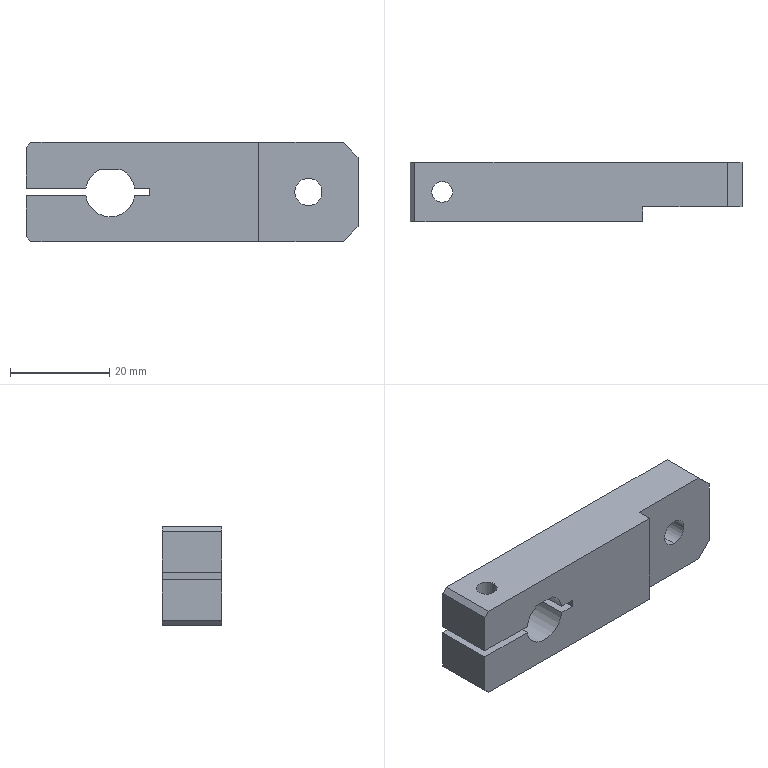Part | NX | features BREP 1 | 1 solid | 31 faces | box 67 x 12 x 20 mm | volume 12717 mm3 | plane 20 | cylinder 11 | commonest cylinder face diameters 10 x5 5.5 x4 4.2 x2
STEP:
#1=CARTESIAN_POINT('',(-22.,0.,-4.3));
#2=VERTEX_POINT('',#1);
#3=CARTESIAN_POINT('',(-32.,0.,-4.3));
#4=VERTEX_POINT('',#3);
#5=CARTESIAN_POINT('',(-27.,0.,-4.3));
#6=DIRECTION('',(0.,0.,-1.));
#7=DIRECTION('',(-1.,0.,0.));
#8=AXIS2_PLACEMENT_3D('',#5,#6,#7);
#9=CIRCLE('',#8,5.);
#10=EDGE_CURVE('',#2,#4,#9,.T.);
#11=ORIENTED_EDGE('',*,*,#10,.F.);
#12=CARTESIAN_POINT('',(-22.,0.,-10.));
#13=VERTEX_POINT('',#12);
#14=CARTESIAN_POINT('',(-22.,0.,-10.));
#15=DIRECTION('',(0.,0.,-1.));
#16=VECTOR('',#15,1000.);
#17=LINE('',#14,#16);
#18=EDGE_CURVE('',#13,#2,#17,.F.);
#19=ORIENTED_EDGE('',*,*,#18,.F.);
#20=CARTESIAN_POINT('',(-32.,0.,-10.));
#21=VERTEX_POINT('',#20);
#22=CARTESIAN_POINT('',(-27.,0.,-10.));
#23=DIRECTION('',(0.,0.,-1.));
#24=DIRECTION('',(-1.,0.,0.));
#25=AXIS2_PLACEMENT_3D('',#22,#23,#24);
#26=CIRCLE('',#25,5.);
#27=EDGE_CURVE('',#13,#21,#26,.T.);
#28=ORIENTED_EDGE('',*,*,#27,.T.);
#29=CARTESIAN_POINT('',(-32.,0.,-10.));
#30=DIRECTION('',(0.,0.,-1.));
#31=VECTOR('',#30,1000.);
#32=LINE('',#29,#31);
#33=EDGE_CURVE('',#21,#4,#32,.F.);
#34=ORIENTED_EDGE('',*,*,#33,.T.);
#35=EDGE_LOOP('',(#11,#19,#28,#34));
#36=FACE_BOUND('',#35,.T.);
#37=CARTESIAN_POINT('',(-27.,0.,-10.));
#38=DIRECTION('',(0.,0.,-1.));
#39=DIRECTION('',(1.,0.,0.));
#40=AXIS2_PLACEMENT_3D('',#37,#38,#39);
#41=CYLINDRICAL_SURFACE('',#40,5.);
#42=ADVANCED_FACE('',(#36),#41,.F.);
#43=CARTESIAN_POINT('',(-24.25,0.,-0.75));
#44=VERTEX_POINT('',#43);
#45=CARTESIAN_POINT('',(-29.75,0.,-0.75));
#46=VERTEX_POINT('',#45);
#47=CARTESIAN_POINT('',(-27.,0.,-0.75));
#48=DIRECTION('',(0.,0.,-1.));
#49=DIRECTION('',(-1.,0.,0.));
#50=AXIS2_PLACEMENT_3D('',#47,#48,#49);
#51=CIRCLE('',#50,2.75);
#52=EDGE_CURVE('',#44,#46,#51,.T.);
#53=ORIENTED_EDGE('',*,*,#52,.F.);
#54=CARTESIAN_POINT('',(-24.25,0.,-4.3));
#55=VERTEX_POINT('',#54);
#56=CARTESIAN_POINT('',(-24.25,0.,-10.));
#57=DIRECTION('',(0.,0.,-1.));
#58=VECTOR('',#57,1000.);
#59=LINE('',#56,#58);
#60=EDGE_CURVE('',#55,#44,#59,.F.);
#61=ORIENTED_EDGE('',*,*,#60,.F.);
#62=CARTESIAN_POINT('',(-29.75,0.,-4.3));
#63=VERTEX_POINT('',#62);
#64=CARTESIAN_POINT('',(-27.,0.,-4.3));
#65=DIRECTION('',(0.,0.,-1.));
#66=DIRECTION('',(-1.,0.,0.));
#67=AXIS2_PLACEMENT_3D('',#64,#65,#66);
#68=CIRCLE('',#67,2.75);
#69=EDGE_CURVE('',#55,#63,#68,.T.);
#70=ORIENTED_EDGE('',*,*,#69,.T.);
#71=CARTESIAN_POINT('',(-29.75,0.,-10.));
#72=DIRECTION('',(0.,0.,-1.));
#73=VECTOR('',#72,1000.);
#74=LINE('',#71,#73);
#75=EDGE_CURVE('',#63,#46,#74,.F.);
#76=ORIENTED_EDGE('',*,*,#75,.T.);
#77=EDGE_LOOP('',(#53,#61,#70,#76));
#78=FACE_BOUND('',#77,.T.);
#79=CARTESIAN_POINT('',(-27.,0.,-10.));
#80=DIRECTION('',(0.,0.,-1.));
#81=DIRECTION('',(1.,0.,0.));
#82=AXIS2_PLACEMENT_3D('',#79,#80,#81);
#83=CYLINDRICAL_SURFACE('',#82,2.75);
#84=ADVANCED_FACE('',(#78),#83,.F.);
#85=CARTESIAN_POINT('',(-29.1,0.,0.75));
#86=VERTEX_POINT('',#85);
#87=CARTESIAN_POINT('',(-24.9,0.,0.75));
#88=VERTEX_POINT('',#87);
#89=CARTESIAN_POINT('',(-27.,0.,0.75));
#90=DIRECTION('',(0.,0.,1.));
#91=DIRECTION('',(1.,0.,0.));
#92=AXIS2_PLACEMENT_3D('',#89,#90,#91);
#93=CIRCLE('',#92,2.1);
#94=EDGE_CURVE('',#86,#88,#93,.T.);
#95=ORIENTED_EDGE('',*,*,#94,.F.);
#96=CARTESIAN_POINT('',(-29.1,0.,10.));
#97=VERTEX_POINT('',#96);
#98=CARTESIAN_POINT('',(-29.1,0.,10.));
#99=DIRECTION('',(0.,0.,1.));
#100=VECTOR('',#99,1000.);
#101=LINE('',#98,#100);
#102=EDGE_CURVE('',#86,#97,#101,.T.);
#103=ORIENTED_EDGE('',*,*,#102,.T.);
#104=CARTESIAN_POINT('',(-24.9,0.,10.));
#105=VERTEX_POINT('',#104);
#106=CARTESIAN_POINT('',(-27.,0.,10.));
#107=DIRECTION('',(0.,0.,1.));
#108=DIRECTION('',(1.,0.,0.));
#109=AXIS2_PLACEMENT_3D('',#106,#107,#108);
#110=CIRCLE('',#109,2.1);
#111=EDGE_CURVE('',#97,#105,#110,.T.);
#112=ORIENTED_EDGE('',*,*,#111,.T.);
#113=CARTESIAN_POINT('',(-24.9,0.,10.));
#114=DIRECTION('',(0.,0.,1.));
#115=VECTOR('',#114,1000.);
#116=LINE('',#113,#115);
#117=EDGE_CURVE('',#88,#105,#116,.T.);
#118=ORIENTED_EDGE('',*,*,#117,.F.);
#119=EDGE_LOOP('',(#95,#103,#112,#118));
#120=FACE_BOUND('',#119,.T.);
#121=CARTESIAN_POINT('',(-27.,0.,10.));
#122=DIRECTION('',(0.,0.,1.));
#123=DIRECTION('',(-1.,0.,0.));
#124=AXIS2_PLACEMENT_3D('',#121,#122,#123);
#125=CYLINDRICAL_SURFACE('',#124,2.1);
#126=ADVANCED_FACE('',(#120),#125,.F.);
#127=CARTESIAN_POINT('',(23.5,-3.,2.75));
#128=VERTEX_POINT('',#127);
#129=CARTESIAN_POINT('',(23.5,-3.,-2.75));
#130=VERTEX_POINT('',#129);
#131=CARTESIAN_POINT('',(23.5,-3.,0.));
#132=DIRECTION('',(0.,-1.,0.));
#133=DIRECTION('',(-1.,0.,0.));
#134=AXIS2_PLACEMENT_3D('',#131,#132,#133);
#135=CIRCLE('',#134,2.75);
#136=EDGE_CURVE('',#128,#130,#135,.T.);
#137=ORIENTED_EDGE('',*,*,#136,.T.);
#138=CARTESIAN_POINT('',(23.5,6.,-2.75));
#139=VERTEX_POINT('',#138);
#140=CARTESIAN_POINT('',(23.5,-6.,-2.75));
#141=DIRECTION('',(0.,1.,0.));
#142=VECTOR('',#141,1000.);
#143=LINE('',#140,#142);
#144=EDGE_CURVE('',#130,#139,#143,.T.);
#145=ORIENTED_EDGE('',*,*,#144,.T.);
#146=CARTESIAN_POINT('',(23.5,6.,2.75));
#147=VERTEX_POINT('',#146);
#148=CARTESIAN_POINT('',(23.5,6.,0.));
#149=DIRECTION('',(0.,1.,0.));
#150=DIRECTION('',(0.,0.,1.));
#151=AXIS2_PLACEMENT_3D('',#148,#149,#150);
#152=CIRCLE('',#151,2.75);
#153=EDGE_CURVE('',#139,#147,#152,.T.);
#154=ORIENTED_EDGE('',*,*,#153,.T.);
#155=CARTESIAN_POINT('',(23.5,-6.,2.75));
#156=DIRECTION('',(0.,1.,0.));
#157=VECTOR('',#156,1000.);
#158=LINE('',#155,#157);
#159=EDGE_CURVE('',#128,#147,#158,.T.);
#160=ORIENTED_EDGE('',*,*,#159,.F.);
#161=EDGE_LOOP('',(#137,#145,#154,#160));
#162=FACE_BOUND('',#161,.T.);
#163=CARTESIAN_POINT('',(23.5,-6.,0.));
#164=DIRECTION('',(0.,1.,0.));
#165=DIRECTION('',(0.,0.,-1.));
#166=AXIS2_PLACEMENT_3D('',#163,#164,#165);
#167=CYLINDRICAL_SURFACE('',#166,2.75);
#168=ADVANCED_FACE('',(#162),#167,.F.);
#169=CARTESIAN_POINT('',(30.5,6.,-10.));
#170=VERTEX_POINT('',#169);
#171=CARTESIAN_POINT('',(-32.5,6.,-10.));
#172=VERTEX_POINT('',#171);
#173=CARTESIAN_POINT('',(-33.5,6.,-10.));
#174=DIRECTION('',(-1.,0.,0.));
#175=VECTOR('',#174,1000.);
#176=LINE('',#173,#175);
#177=EDGE_CURVE('',#170,#172,#176,.T.);
#178=ORIENTED_EDGE('',*,*,#177,.F.);
#179=CARTESIAN_POINT('',(30.5,-3.,-10.));
#180=VERTEX_POINT('',#179);
#181=CARTESIAN_POINT('',(30.5,6.,-10.));
#182=DIRECTION('',(0.,-1.,0.));
#183=VECTOR('',#182,1000.);
#184=LINE('',#181,#183);
#185=EDGE_CURVE('',#170,#180,#184,.T.);
#186=ORIENTED_EDGE('',*,*,#185,.T.);
#187=CARTESIAN_POINT('',(13.5,-3.,-10.));
#188=VERTEX_POINT('',#187);
#189=CARTESIAN_POINT('',(33.5,-3.,-10.));
#190=DIRECTION('',(-1.,0.,0.));
#191=VECTOR('',#190,1000.);
#192=LINE('',#189,#191);
#193=EDGE_CURVE('',#180,#188,#192,.T.);
#194=ORIENTED_EDGE('',*,*,#193,.T.);
#195=CARTESIAN_POINT('',(13.5,-6.,-10.));
#196=VERTEX_POINT('',#195);
#197=CARTESIAN_POINT('',(13.5,-6.,-10.));
#198=DIRECTION('',(0.,-1.,0.));
#199=VECTOR('',#198,1000.);
#200=LINE('',#197,#199);
#201=EDGE_CURVE('',#188,#196,#200,.T.);
#202=ORIENTED_EDGE('',*,*,#201,.T.);
#203=CARTESIAN_POINT('',(-32.5,-6.,-10.));
#204=VERTEX_POINT('',#203);
#205=CARTESIAN_POINT('',(-33.5,-6.,-10.));
#206=DIRECTION('',(-1.,0.,0.));
#207=VECTOR('',#206,1000.);
#208=LINE('',#205,#207);
#209=EDGE_CURVE('',#196,#204,#208,.T.);
#210=ORIENTED_EDGE('',*,*,#209,.T.);
#211=CARTESIAN_POINT('',(-32.5,6.,-10.));
#212=DIRECTION('',(0.,1.,0.));
#213=VECTOR('',#212,1000.);
#214=LINE('',#211,#213);
#215=EDGE_CURVE('',#204,#172,#214,.T.);
#216=ORIENTED_EDGE('',*,*,#215,.T.);
#217=EDGE_LOOP('',(#178,#186,#194,#202,#210,#216));
#218=FACE_BOUND('',#217,.T.);
#219=CARTESIAN_POINT('',(-27.,0.,-10.));
#220=DIRECTION('',(0.,0.,-1.));
#221=DIRECTION('',(-1.,0.,0.));
#222=AXIS2_PLACEMENT_3D('',#219,#220,#221);
#223=CIRCLE('',#222,5.);
#224=EDGE_CURVE('',#21,#13,#223,.T.);
#225=ORIENTED_EDGE('',*,*,#224,.F.);
#226=ORIENTED_EDGE('',*,*,#27,.F.);
#227=EDGE_LOOP('',(#225,#226));
#228=FACE_BOUND('',#227,.T.);
#229=CARTESIAN_POINT('',(-33.5,6.,-10.));
#230=DIRECTION('',(0.,0.,1.));
#231=DIRECTION('',(-1.,0.,0.));
#232=AXIS2_PLACEMENT_3D('',#229,#230,#231);
#233=PLANE('',#232);
#234=ADVANCED_FACE('',(#218,#228),#233,.F.);
#235=CARTESIAN_POINT('',(13.5,-3.,10.));
#236=VERTEX_POINT('',#235);
#237=CARTESIAN_POINT('',(30.5,-3.,10.));
#238=VERTEX_POINT('',#237);
#239=CARTESIAN_POINT('',(-33.5,-3.,10.));
#240=DIRECTION('',(1.,0.,0.));
#241=VECTOR('',#240,1000.);
#242=LINE('',#239,#241);
#243=EDGE_CURVE('',#236,#238,#242,.T.);
#244=ORIENTED_EDGE('',*,*,#243,.T.);
#245=CARTESIAN_POINT('',(30.5,6.,10.));
#246=VERTEX_POINT('',#245);
#247=CARTESIAN_POINT('',(30.5,6.,10.));
#248=DIRECTION('',(0.,1.,0.));
#249=VECTOR('',#248,1000.);
#250=LINE('',#247,#249);
#251=EDGE_CURVE('',#238,#246,#250,.T.);
#252=ORIENTED_EDGE('',*,*,#251,.T.);
#253=CARTESIAN_POINT('',(-32.5,6.,10.));
#254=VERTEX_POINT('',#253);
#255=CARTESIAN_POINT('',(-33.5,6.,10.));
#256=DIRECTION('',(1.,0.,0.));
#257=VECTOR('',#256,1000.);
#258=LINE('',#255,#257);
#259=EDGE_CURVE('',#254,#246,#258,.T.);
#260=ORIENTED_EDGE('',*,*,#259,.F.);
#261=CARTESIAN_POINT('',(-32.5,-6.,10.));
#262=VERTEX_POINT('',#261);
#263=CARTESIAN_POINT('',(-32.5,6.,10.));
#264=DIRECTION('',(0.,-1.,0.));
#265=VECTOR('',#264,1000.);
#266=LINE('',#263,#265);
#267=EDGE_CURVE('',#254,#262,#266,.T.);
#268=ORIENTED_EDGE('',*,*,#267,.T.);
#269=CARTESIAN_POINT('',(13.5,-6.,10.));
#270=VERTEX_POINT('',#269);
#271=CARTESIAN_POINT('',(-33.5,-6.,10.));
#272=DIRECTION('',(1.,0.,0.));
#273=VECTOR('',#272,1000.);
#274=LINE('',#271,#273);
#275=EDGE_CURVE('',#262,#270,#274,.T.);
#276=ORIENTED_EDGE('',*,*,#275,.T.);
#277=CARTESIAN_POINT('',(13.5,6.,10.));
#278=DIRECTION('',(0.,1.,0.));
#279=VECTOR('',#278,1000.);
#280=LINE('',#277,#279);
#281=EDGE_CURVE('',#270,#236,#280,.T.);
#282=ORIENTED_EDGE('',*,*,#281,.T.);
#283=EDGE_LOOP('',(#244,#252,#260,#268,#276,#282));
#284=FACE_BOUND('',#283,.T.);
#285=CARTESIAN_POINT('',(-27.,0.,10.));
#286=DIRECTION('',(0.,0.,1.));
#287=DIRECTION('',(1.,0.,0.));
#288=AXIS2_PLACEMENT_3D('',#285,#286,#287);
#289=CIRCLE('',#288,2.1);
#290=EDGE_CURVE('',#105,#97,#289,.T.);
#291=ORIENTED_EDGE('',*,*,#290,.F.);
#292=ORIENTED_EDGE('',*,*,#111,.F.);
#293=EDGE_LOOP('',(#291,#292));
#294=FACE_BOUND('',#293,.T.);
#295=CARTESIAN_POINT('',(-33.5,6.,10.));
#296=DIRECTION('',(0.,0.,-1.));
#297=DIRECTION('',(1.,0.,0.));
#298=AXIS2_PLACEMENT_3D('',#295,#296,#297);
#299=PLANE('',#298);
#300=ADVANCED_FACE('',(#284,#294),#299,.F.);
#301=CARTESIAN_POINT('',(-33.5,-6.,-9.));
#302=VERTEX_POINT('',#301);
#303=CARTESIAN_POINT('',(-33.5,-6.,-0.75));
#304=VERTEX_POINT('',#303);
#305=CARTESIAN_POINT('',(-33.5,-6.,-10.));
#306=DIRECTION('',(0.,0.,1.));
#307=VECTOR('',#306,1000.);
#308=LINE('',#305,#307);
#309=EDGE_CURVE('',#302,#304,#308,.T.);
#310=ORIENTED_EDGE('',*,*,#309,.T.);
#311=CARTESIAN_POINT('',(-33.5,6.,-0.75));
#312=VERTEX_POINT('',#311);
#313=CARTESIAN_POINT('',(-33.5,6.,-0.75));
#314=DIRECTION('',(0.,-1.,0.));
#315=VECTOR('',#314,1000.);
#316=LINE('',#313,#315);
#317=EDGE_CURVE('',#312,#304,#316,.T.);
#318=ORIENTED_EDGE('',*,*,#317,.F.);
#319=CARTESIAN_POINT('',(-33.5,6.,-9.));
#320=VERTEX_POINT('',#319);
#321=CARTESIAN_POINT('',(-33.5,6.,-10.));
#322=DIRECTION('',(0.,0.,1.));
#323=VECTOR('',#322,1000.);
#324=LINE('',#321,#323);
#325=EDGE_CURVE('',#320,#312,#324,.T.);
#326=ORIENTED_EDGE('',*,*,#325,.F.);
#327=CARTESIAN_POINT('',(-33.5,6.,-9.));
#328=DIRECTION('',(0.,-1.,0.));
#329=VECTOR('',#328,1000.);
#330=LINE('',#327,#329);
#331=EDGE_CURVE('',#320,#302,#330,.T.);
#332=ORIENTED_EDGE('',*,*,#331,.T.);
#333=EDGE_LOOP('',(#310,#318,#326,#332));
#334=FACE_BOUND('',#333,.T.);
#335=CARTESIAN_POINT('',(-33.5,6.,-10.));
#336=DIRECTION('',(1.,0.,0.));
#337=DIRECTION('',(0.,0.,1.));
#338=AXIS2_PLACEMENT_3D('',#335,#336,#337);
#339=PLANE('',#338);
#340=ADVANCED_FACE('',(#334),#339,.F.);
#341=CARTESIAN_POINT('',(-11.557,6.,-0.75));
#342=VERTEX_POINT('',#341);
#343=CARTESIAN_POINT('',(-21.443,6.,-0.75));
#344=VERTEX_POINT('',#343);
#345=CARTESIAN_POINT('',(-16.5,6.,0.));
#346=DIRECTION('',(0.,1.,0.));
#347=DIRECTION('',(0.,0.,1.));
#348=AXIS2_PLACEMENT_3D('',#345,#346,#347);
#349=CIRCLE('',#348,5.);
#350=EDGE_CURVE('',#342,#344,#349,.T.);
#351=ORIENTED_EDGE('',*,*,#350,.T.);
#352=CARTESIAN_POINT('',(-21.443,-6.,-0.75));
#353=VERTEX_POINT('',#352);
#354=CARTESIAN_POINT('',(-21.443,-6.,-0.75));
#355=DIRECTION('',(0.,-1.,0.));
#356=VECTOR('',#355,1000.);
#357=LINE('',#354,#356);
#358=EDGE_CURVE('',#344,#353,#357,.T.);
#359=ORIENTED_EDGE('',*,*,#358,.T.);
#360=CARTESIAN_POINT('',(-11.557,-6.,-0.75));
#361=VERTEX_POINT('',#360);
#362=CARTESIAN_POINT('',(-16.5,-6.,0.));
#363=DIRECTION('',(0.,1.,0.));
#364=DIRECTION('',(0.,0.,1.));
#365=AXIS2_PLACEMENT_3D('',#362,#363,#364);
#366=CIRCLE('',#365,5.);
#367=EDGE_CURVE('',#361,#353,#366,.T.);
#368=ORIENTED_EDGE('',*,*,#367,.F.);
#369=CARTESIAN_POINT('',(-11.557,-6.,-0.75));
#370=DIRECTION('',(0.,1.,0.));
#371=VECTOR('',#370,1000.);
#372=LINE('',#369,#371);
#373=EDGE_CURVE('',#361,#342,#372,.T.);
#374=ORIENTED_EDGE('',*,*,#373,.T.);
#375=EDGE_LOOP('',(#351,#359,#368,#374));
#376=FACE_BOUND('',#375,.T.);
#377=CARTESIAN_POINT('',(-16.5,-6.,0.));
#378=DIRECTION('',(0.,1.,0.));
#379=DIRECTION('',(0.,0.,-1.));
#380=AXIS2_PLACEMENT_3D('',#377,#378,#379);
#381=CYLINDRICAL_SURFACE('',#380,5.);
#382=ADVANCED_FACE('',(#376),#381,.F.);
#383=CARTESIAN_POINT('',(-14.321,6.,4.5));
#384=VERTEX_POINT('',#383);
#385=CARTESIAN_POINT('',(-11.557,6.,0.75));
#386=VERTEX_POINT('',#385);
#387=CARTESIAN_POINT('',(-16.5,6.,0.));
#388=DIRECTION('',(0.,1.,0.));
#389=DIRECTION('',(0.,0.,1.));
#390=AXIS2_PLACEMENT_3D('',#387,#388,#389);
#391=CIRCLE('',#390,5.);
#392=EDGE_CURVE('',#384,#386,#391,.T.);
#393=ORIENTED_EDGE('',*,*,#392,.T.);
#394=CARTESIAN_POINT('',(-11.557,-6.,0.75));
#395=VERTEX_POINT('',#394);
#396=CARTESIAN_POINT('',(-11.557,-6.,0.75));
#397=DIRECTION('',(0.,-1.,0.));
#398=VECTOR('',#397,1000.);
#399=LINE('',#396,#398);
#400=EDGE_CURVE('',#386,#395,#399,.T.);
#401=ORIENTED_EDGE('',*,*,#400,.T.);
#402=CARTESIAN_POINT('',(-14.321,-6.,4.5));
#403=VERTEX_POINT('',#402);
#404=CARTESIAN_POINT('',(-16.5,-6.,0.));
#405=DIRECTION('',(0.,1.,0.));
#406=DIRECTION('',(0.,0.,1.));
#407=AXIS2_PLACEMENT_3D('',#404,#405,#406);
#408=CIRCLE('',#407,5.);
#409=EDGE_CURVE('',#403,#395,#408,.T.);
#410=ORIENTED_EDGE('',*,*,#409,.F.);
#411=CARTESIAN_POINT('',(-14.321,-6.,4.5));
#412=DIRECTION('',(0.,1.,0.));
#413=VECTOR('',#412,1000.);
#414=LINE('',#411,#413);
#415=EDGE_CURVE('',#403,#384,#414,.T.);
#416=ORIENTED_EDGE('',*,*,#415,.T.);
#417=EDGE_LOOP('',(#393,#401,#410,#416));
#418=FACE_BOUND('',#417,.T.);
#419=CARTESIAN_POINT('',(-16.5,-6.,0.));
#420=DIRECTION('',(0.,1.,0.));
#421=DIRECTION('',(0.,0.,-1.));
#422=AXIS2_PLACEMENT_3D('',#419,#420,#421);
#423=CYLINDRICAL_SURFACE('',#422,5.);
#424=ADVANCED_FACE('',(#418),#423,.F.);
#425=CARTESIAN_POINT('',(33.5,6.,7.));
#426=VERTEX_POINT('',#425);
#427=CARTESIAN_POINT('',(33.5,6.,-7.));
#428=VERTEX_POINT('',#427);
#429=CARTESIAN_POINT('',(33.5,6.,-10.));
#430=DIRECTION('',(0.,0.,-1.));
#431=VECTOR('',#430,1000.);
#432=LINE('',#429,#431);
#433=EDGE_CURVE('',#426,#428,#432,.T.);
#434=ORIENTED_EDGE('',*,*,#433,.F.);
#435=CARTESIAN_POINT('',(33.5,-3.,7.));
#436=VERTEX_POINT('',#435);
#437=CARTESIAN_POINT('',(33.5,6.,7.));
#438=DIRECTION('',(0.,-1.,0.));
#439=VECTOR('',#438,1000.);
#440=LINE('',#437,#439);
#441=EDGE_CURVE('',#426,#436,#440,.T.);
#442=ORIENTED_EDGE('',*,*,#441,.T.);
#443=CARTESIAN_POINT('',(33.5,-3.,-7.));
#444=VERTEX_POINT('',#443);
#445=CARTESIAN_POINT('',(33.5,-3.,-10.));
#446=DIRECTION('',(0.,0.,1.));
#447=VECTOR('',#446,1000.);
#448=LINE('',#445,#447);
#449=EDGE_CURVE('',#444,#436,#448,.T.);
#450=ORIENTED_EDGE('',*,*,#449,.F.);
#451=CARTESIAN_POINT('',(33.5,6.,-7.));
#452=DIRECTION('',(0.,1.,0.));
#453=VECTOR('',#452,1000.);
#454=LINE('',#451,#453);
#455=EDGE_CURVE('',#444,#428,#454,.T.);
#456=ORIENTED_EDGE('',*,*,#455,.T.);
#457=EDGE_LOOP('',(#434,#442,#450,#456));
#458=FACE_BOUND('',#457,.T.);
#459=CARTESIAN_POINT('',(33.5,6.,-10.));
#460=DIRECTION('',(-1.,0.,0.));
#461=DIRECTION('',(0.,0.,-1.));
#462=AXIS2_PLACEMENT_3D('',#459,#460,#461);
#463=PLANE('',#462);
#464=ADVANCED_FACE('',(#458),#463,.F.);
#465=CARTESIAN_POINT('',(-33.5,6.,0.75));
#466=VERTEX_POINT('',#465);
#467=CARTESIAN_POINT('',(-33.5,6.,9.));
#468=VERTEX_POINT('',#467);
#469=CARTESIAN_POINT('',(-33.5,6.,-10.));
#470=DIRECTION('',(0.,0.,1.));
#471=VECTOR('',#470,1000.);
#472=LINE('',#469,#471);
#473=EDGE_CURVE('',#466,#468,#472,.T.);
#474=ORIENTED_EDGE('',*,*,#473,.F.);
#475=CARTESIAN_POINT('',(-33.5,-6.,0.75));
#476=VERTEX_POINT('',#475);
#477=CARTESIAN_POINT('',(-33.5,6.,0.75));
#478=DIRECTION('',(0.,-1.,0.));
#479=VECTOR('',#478,1000.);
#480=LINE('',#477,#479);
#481=EDGE_CURVE('',#466,#476,#480,.T.);
#482=ORIENTED_EDGE('',*,*,#481,.T.);
#483=CARTESIAN_POINT('',(-33.5,-6.,9.));
#484=VERTEX_POINT('',#483);
#485=CARTESIAN_POINT('',(-33.5,-6.,-10.));
#486=DIRECTION('',(0.,0.,1.));
#487=VECTOR('',#486,1000.);
#488=LINE('',#485,#487);
#489=EDGE_CURVE('',#476,#484,#488,.T.);
#490=ORIENTED_EDGE('',*,*,#489,.T.);
#491=CARTESIAN_POINT('',(-33.5,6.,9.));
#492=DIRECTION('',(0.,1.,0.));
#493=VECTOR('',#492,1000.);
#494=LINE('',#491,#493);
#495=EDGE_CURVE('',#484,#468,#494,.T.);
#496=ORIENTED_EDGE('',*,*,#495,.T.);
#497=EDGE_LOOP('',(#474,#482,#490,#496));
#498=FACE_BOUND('',#497,.T.);
#499=CARTESIAN_POINT('',(-33.5,6.,-10.));
#500=DIRECTION('',(1.,0.,0.));
#501=DIRECTION('',(0.,0.,1.));
#502=AXIS2_PLACEMENT_3D('',#499,#500,#501);
#503=PLANE('',#502);
#504=ADVANCED_FACE('',(#498),#503,.F.);
#505=ORIENTED_EDGE('',*,*,#259,.T.);
#506=CARTESIAN_POINT('',(20.25,6.,20.25));
#507=DIRECTION('',(0.7071,0.,-0.7071));
#508=VECTOR('',#507,1000.);
#509=LINE('',#506,#508);
#510=EDGE_CURVE('',#246,#426,#509,.T.);
#511=ORIENTED_EDGE('',*,*,#510,.T.);
#512=ORIENTED_EDGE('',*,*,#433,.T.);
#513=CARTESIAN_POINT('',(20.25,6.,-20.25));
#514=DIRECTION('',(-0.7071,0.,-0.7071));
#515=VECTOR('',#514,1000.);
#516=LINE('',#513,#515);
#517=EDGE_CURVE('',#428,#170,#516,.T.);
#518=ORIENTED_EDGE('',*,*,#517,.T.);
#519=ORIENTED_EDGE('',*,*,#177,.T.);
#520=CARTESIAN_POINT('',(-21.25,6.,-21.25));
#521=DIRECTION('',(-0.7071,0.,0.7071));
#522=VECTOR('',#521,1000.);
#523=LINE('',#520,#522);
#524=EDGE_CURVE('',#172,#320,#523,.T.);
#525=ORIENTED_EDGE('',*,*,#524,.T.);
#526=ORIENTED_EDGE('',*,*,#325,.T.);
#527=CARTESIAN_POINT('',(-33.5,6.,-0.75));
#528=DIRECTION('',(1.,0.,0.));
#529=VECTOR('',#528,1000.);
#530=LINE('',#527,#529);
#531=EDGE_CURVE('',#312,#344,#530,.T.);
#532=ORIENTED_EDGE('',*,*,#531,.T.);
#533=ORIENTED_EDGE('',*,*,#350,.F.);
#534=CARTESIAN_POINT('',(-8.5,6.,-0.75));
#535=VERTEX_POINT('',#534);
#536=CARTESIAN_POINT('',(-33.5,6.,-0.75));
#537=DIRECTION('',(1.,0.,0.));
#538=VECTOR('',#537,1000.);
#539=LINE('',#536,#538);
#540=EDGE_CURVE('',#342,#535,#539,.T.);
#541=ORIENTED_EDGE('',*,*,#540,.T.);
#542=CARTESIAN_POINT('',(-8.5,6.,0.75));
#543=VERTEX_POINT('',#542);
#544=CARTESIAN_POINT('',(-8.5,6.,-0.75));
#545=DIRECTION('',(0.,0.,1.));
#546=VECTOR('',#545,1000.);
#547=LINE('',#544,#546);
#548=EDGE_CURVE('',#535,#543,#547,.T.);
#549=ORIENTED_EDGE('',*,*,#548,.T.);
#550=CARTESIAN_POINT('',(-33.5,6.,0.75));
#551=DIRECTION('',(-1.,0.,0.));
#552=VECTOR('',#551,1000.);
#553=LINE('',#550,#552);
#554=EDGE_CURVE('',#543,#386,#553,.T.);
#555=ORIENTED_EDGE('',*,*,#554,.T.);
#556=ORIENTED_EDGE('',*,*,#392,.F.);
#557=CARTESIAN_POINT('',(-18.679,6.,4.5));
#558=VERTEX_POINT('',#557);
#559=CARTESIAN_POINT('',(-18.679,6.,4.5));
#560=DIRECTION('',(1.,0.,0.));
#561=VECTOR('',#560,1000.);
#562=LINE('',#559,#561);
#563=EDGE_CURVE('',#558,#384,#562,.T.);
#564=ORIENTED_EDGE('',*,*,#563,.F.);
#565=CARTESIAN_POINT('',(-21.443,6.,0.75));
#566=VERTEX_POINT('',#565);
#567=CARTESIAN_POINT('',(-16.5,6.,0.));
#568=DIRECTION('',(0.,1.,0.));
#569=DIRECTION('',(0.,0.,1.));
#570=AXIS2_PLACEMENT_3D('',#567,#568,#569);
#571=CIRCLE('',#570,5.);
#572=EDGE_CURVE('',#566,#558,#571,.T.);
#573=ORIENTED_EDGE('',*,*,#572,.F.);
#574=CARTESIAN_POINT('',(-33.5,6.,0.75));
#575=DIRECTION('',(-1.,0.,0.));
#576=VECTOR('',#575,1000.);
#577=LINE('',#574,#576);
#578=EDGE_CURVE('',#566,#466,#577,.T.);
#579=ORIENTED_EDGE('',*,*,#578,.T.);
#580=ORIENTED_EDGE('',*,*,#473,.T.);
#581=CARTESIAN_POINT('',(-21.25,6.,21.25));
#582=DIRECTION('',(0.7071,0.,0.7071));
#583=VECTOR('',#582,1000.);
#584=LINE('',#581,#583);
#585=EDGE_CURVE('',#468,#254,#584,.T.);
#586=ORIENTED_EDGE('',*,*,#585,.T.);
#587=EDGE_LOOP('',(#505,#511,#512,#518,#519,#525,#526,#532,#533,#541,#549,#555,#556,#564,#573,#579,#580,#586));
#588=FACE_BOUND('',#587,.T.);
#589=CARTESIAN_POINT('',(23.5,6.,0.));
#590=DIRECTION('',(0.,1.,0.));
#591=DIRECTION('',(0.,0.,1.));
#592=AXIS2_PLACEMENT_3D('',#589,#590,#591);
#593=CIRCLE('',#592,2.75);
#594=EDGE_CURVE('',#147,#139,#593,.T.);
#595=ORIENTED_EDGE('',*,*,#594,.F.);
#596=ORIENTED_EDGE('',*,*,#153,.F.);
#597=EDGE_LOOP('',(#595,#596));
#598=FACE_BOUND('',#597,.T.);
#599=CARTESIAN_POINT('',(0.,6.,0.));
#600=DIRECTION('',(0.,1.,0.));
#601=DIRECTION('',(0.,0.,-1.));
#602=AXIS2_PLACEMENT_3D('',#599,#600,#601);
#603=PLANE('',#602);
#604=ADVANCED_FACE('',(#588,#598),#603,.T.);
#605=ORIENTED_EDGE('',*,*,#367,.T.);
#606=CARTESIAN_POINT('',(-33.5,-6.,-0.75));
#607=DIRECTION('',(1.,0.,0.));
#608=VECTOR('',#607,1000.);
#609=LINE('',#606,#608);
#610=EDGE_CURVE('',#304,#353,#609,.T.);
#611=ORIENTED_EDGE('',*,*,#610,.F.);
#612=ORIENTED_EDGE('',*,*,#309,.F.);
#613=CARTESIAN_POINT('',(-33.5,-6.,-9.));
#614=DIRECTION('',(0.7071,0.,-0.7071));
#615=VECTOR('',#614,1000.);
#616=LINE('',#613,#615);
#617=EDGE_CURVE('',#302,#204,#616,.T.);
#618=ORIENTED_EDGE('',*,*,#617,.T.);
#619=ORIENTED_EDGE('',*,*,#209,.F.);
#620=CARTESIAN_POINT('',(13.5,-6.,-10.));
#621=DIRECTION('',(0.,0.,1.));
#622=VECTOR('',#621,1000.);
#623=LINE('',#620,#622);
#624=EDGE_CURVE('',#196,#270,#623,.T.);
#625=ORIENTED_EDGE('',*,*,#624,.T.);
#626=ORIENTED_EDGE('',*,*,#275,.F.);
#627=CARTESIAN_POINT('',(-32.5,-6.,10.));
#628=DIRECTION('',(-0.7071,0.,-0.7071));
#629=VECTOR('',#628,1000.);
#630=LINE('',#627,#629);
#631=EDGE_CURVE('',#262,#484,#630,.T.);
#632=ORIENTED_EDGE('',*,*,#631,.T.);
#633=ORIENTED_EDGE('',*,*,#489,.F.);
#634=CARTESIAN_POINT('',(-21.443,-6.,0.75));
#635=VERTEX_POINT('',#634);
#636=CARTESIAN_POINT('',(-33.5,-6.,0.75));
#637=DIRECTION('',(-1.,0.,0.));
#638=VECTOR('',#637,1000.);
#639=LINE('',#636,#638);
#640=EDGE_CURVE('',#635,#476,#639,.T.);
#641=ORIENTED_EDGE('',*,*,#640,.F.);
#642=CARTESIAN_POINT('',(-18.679,-6.,4.5));
#643=VERTEX_POINT('',#642);
#644=CARTESIAN_POINT('',(-16.5,-6.,0.));
#645=DIRECTION('',(0.,1.,0.));
#646=DIRECTION('',(0.,0.,1.));
#647=AXIS2_PLACEMENT_3D('',#644,#645,#646);
#648=CIRCLE('',#647,5.);
#649=EDGE_CURVE('',#635,#643,#648,.T.);
#650=ORIENTED_EDGE('',*,*,#649,.T.);
#651=CARTESIAN_POINT('',(-18.679,-6.,4.5));
#652=DIRECTION('',(1.,0.,0.));
#653=VECTOR('',#652,1000.);
#654=LINE('',#651,#653);
#655=EDGE_CURVE('',#643,#403,#654,.T.);
#656=ORIENTED_EDGE('',*,*,#655,.T.);
#657=ORIENTED_EDGE('',*,*,#409,.T.);
#658=CARTESIAN_POINT('',(-8.5,-6.,0.75));
#659=VERTEX_POINT('',#658);
#660=CARTESIAN_POINT('',(-33.5,-6.,0.75));
#661=DIRECTION('',(-1.,0.,0.));
#662=VECTOR('',#661,1000.);
#663=LINE('',#660,#662);
#664=EDGE_CURVE('',#659,#395,#663,.T.);
#665=ORIENTED_EDGE('',*,*,#664,.F.);
#666=CARTESIAN_POINT('',(-8.5,-6.,-0.75));
#667=VERTEX_POINT('',#666);
#668=CARTESIAN_POINT('',(-8.5,-6.,-0.75));
#669=DIRECTION('',(0.,0.,1.));
#670=VECTOR('',#669,1000.);
#671=LINE('',#668,#670);
#672=EDGE_CURVE('',#667,#659,#671,.T.);
#673=ORIENTED_EDGE('',*,*,#672,.F.);
#674=CARTESIAN_POINT('',(-33.5,-6.,-0.75));
#675=DIRECTION('',(1.,0.,0.));
#676=VECTOR('',#675,1000.);
#677=LINE('',#674,#676);
#678=EDGE_CURVE('',#361,#667,#677,.T.);
#679=ORIENTED_EDGE('',*,*,#678,.F.);
#680=EDGE_LOOP('',(#605,#611,#612,#618,#619,#625,#626,#632,#633,#641,#650,#656,#657,#665,#673,#679));
#681=FACE_BOUND('',#680,.T.);
#682=CARTESIAN_POINT('',(0.,-6.,0.));
#683=DIRECTION('',(0.,1.,0.));
#684=DIRECTION('',(0.,0.,-1.));
#685=AXIS2_PLACEMENT_3D('',#682,#683,#684);
#686=PLANE('',#685);
#687=ADVANCED_FACE('',(#681),#686,.F.);
#688=ORIENTED_EDGE('',*,*,#649,.F.);
#689=CARTESIAN_POINT('',(-21.443,-6.,0.75));
#690=DIRECTION('',(0.,1.,0.));
#691=VECTOR('',#690,1000.);
#692=LINE('',#689,#691);
#693=EDGE_CURVE('',#635,#566,#692,.T.);
#694=ORIENTED_EDGE('',*,*,#693,.T.);
#695=ORIENTED_EDGE('',*,*,#572,.T.);
#696=CARTESIAN_POINT('',(-18.679,-6.,4.5));
#697=DIRECTION('',(0.,1.,0.));
#698=VECTOR('',#697,1000.);
#699=LINE('',#696,#698);
#700=EDGE_CURVE('',#643,#558,#699,.T.);
#701=ORIENTED_EDGE('',*,*,#700,.F.);
#702=EDGE_LOOP('',(#688,#694,#695,#701));
#703=FACE_BOUND('',#702,.T.);
#704=CARTESIAN_POINT('',(-16.5,-6.,0.));
#705=DIRECTION('',(0.,1.,0.));
#706=DIRECTION('',(0.,0.,-1.));
#707=AXIS2_PLACEMENT_3D('',#704,#705,#706);
#708=CYLINDRICAL_SURFACE('',#707,5.);
#709=ADVANCED_FACE('',(#703),#708,.F.);
#710=ORIENTED_EDGE('',*,*,#563,.T.);
#711=ORIENTED_EDGE('',*,*,#415,.F.);
#712=ORIENTED_EDGE('',*,*,#655,.F.);
#713=ORIENTED_EDGE('',*,*,#700,.T.);
#714=EDGE_LOOP('',(#710,#711,#712,#713));
#715=FACE_BOUND('',#714,.T.);
#716=CARTESIAN_POINT('',(-18.679,-6.,4.5));
#717=DIRECTION('',(0.,0.,1.));
#718=DIRECTION('',(-1.,0.,0.));
#719=AXIS2_PLACEMENT_3D('',#716,#717,#718);
#720=PLANE('',#719);
#721=ADVANCED_FACE('',(#715),#720,.F.);
#722=ORIENTED_EDGE('',*,*,#144,.F.);
#723=CARTESIAN_POINT('',(23.5,-3.,0.));
#724=DIRECTION('',(0.,-1.,0.));
#725=DIRECTION('',(-1.,0.,0.));
#726=AXIS2_PLACEMENT_3D('',#723,#724,#725);
#727=CIRCLE('',#726,2.75);
#728=EDGE_CURVE('',#130,#128,#727,.T.);
#729=ORIENTED_EDGE('',*,*,#728,.T.);
#730=ORIENTED_EDGE('',*,*,#159,.T.);
#731=ORIENTED_EDGE('',*,*,#594,.T.);
#732=EDGE_LOOP('',(#722,#729,#730,#731));
#733=FACE_BOUND('',#732,.T.);
#734=CARTESIAN_POINT('',(23.5,-6.,0.));
#735=DIRECTION('',(0.,1.,0.));
#736=DIRECTION('',(0.,0.,-1.));
#737=AXIS2_PLACEMENT_3D('',#734,#735,#736);
#738=CYLINDRICAL_SURFACE('',#737,2.75);
#739=ADVANCED_FACE('',(#733),#738,.F.);
#740=ORIENTED_EDGE('',*,*,#624,.F.);
#741=ORIENTED_EDGE('',*,*,#201,.F.);
#742=CARTESIAN_POINT('',(13.5,-3.,-10.));
#743=DIRECTION('',(0.,0.,1.));
#744=VECTOR('',#743,1000.);
#745=LINE('',#742,#744);
#746=EDGE_CURVE('',#188,#236,#745,.T.);
#747=ORIENTED_EDGE('',*,*,#746,.T.);
#748=ORIENTED_EDGE('',*,*,#281,.F.);
#749=EDGE_LOOP('',(#740,#741,#747,#748));
#750=FACE_BOUND('',#749,.T.);
#751=CARTESIAN_POINT('',(13.5,-6.,-10.));
#752=DIRECTION('',(-1.,0.,0.));
#753=DIRECTION('',(0.,0.,-1.));
#754=AXIS2_PLACEMENT_3D('',#751,#752,#753);
#755=PLANE('',#754);
#756=ADVANCED_FACE('',(#750),#755,.F.);
#757=ORIENTED_EDGE('',*,*,#136,.F.);
#758=ORIENTED_EDGE('',*,*,#728,.F.);
#759=EDGE_LOOP('',(#757,#758));
#760=FACE_BOUND('',#759,.T.);
#761=ORIENTED_EDGE('',*,*,#449,.T.);
#762=CARTESIAN_POINT('',(33.5,-3.,7.));
#763=DIRECTION('',(-0.7071,0.,0.7071));
#764=VECTOR('',#763,1000.);
#765=LINE('',#762,#764);
#766=EDGE_CURVE('',#436,#238,#765,.T.);
#767=ORIENTED_EDGE('',*,*,#766,.T.);
#768=ORIENTED_EDGE('',*,*,#243,.F.);
#769=ORIENTED_EDGE('',*,*,#746,.F.);
#770=ORIENTED_EDGE('',*,*,#193,.F.);
#771=CARTESIAN_POINT('',(30.5,-3.,-10.));
#772=DIRECTION('',(0.7071,0.,0.7071));
#773=VECTOR('',#772,1000.);
#774=LINE('',#771,#773);
#775=EDGE_CURVE('',#180,#444,#774,.T.);
#776=ORIENTED_EDGE('',*,*,#775,.T.);
#777=EDGE_LOOP('',(#761,#767,#768,#769,#770,#776));
#778=FACE_BOUND('',#777,.T.);
#779=CARTESIAN_POINT('',(33.5,-3.,-10.));
#780=DIRECTION('',(0.,1.,0.));
#781=DIRECTION('',(1.,0.,0.));
#782=AXIS2_PLACEMENT_3D('',#779,#780,#781);
#783=PLANE('',#782);
#784=ADVANCED_FACE('',(#760,#778),#783,.F.);
#785=ORIENTED_EDGE('',*,*,#585,.F.);
#786=ORIENTED_EDGE('',*,*,#495,.F.);
#787=ORIENTED_EDGE('',*,*,#631,.F.);
#788=ORIENTED_EDGE('',*,*,#267,.F.);
#789=EDGE_LOOP('',(#785,#786,#787,#788));
#790=FACE_BOUND('',#789,.T.);
#791=CARTESIAN_POINT('',(-32.5,6.,10.));
#792=DIRECTION('',(0.7071,0.,-0.7071));
#793=DIRECTION('',(0.,1.,0.));
#794=AXIS2_PLACEMENT_3D('',#791,#792,#793);
#795=PLANE('',#794);
#796=ADVANCED_FACE('',(#790),#795,.F.);
#797=ORIENTED_EDGE('',*,*,#524,.F.);
#798=ORIENTED_EDGE('',*,*,#215,.F.);
#799=ORIENTED_EDGE('',*,*,#617,.F.);
#800=ORIENTED_EDGE('',*,*,#331,.F.);
#801=EDGE_LOOP('',(#797,#798,#799,#800));
#802=FACE_BOUND('',#801,.T.);
#803=CARTESIAN_POINT('',(-33.5,6.,-9.));
#804=DIRECTION('',(0.7071,0.,0.7071));
#805=DIRECTION('',(0.,1.,0.));
#806=AXIS2_PLACEMENT_3D('',#803,#804,#805);
#807=PLANE('',#806);
#808=ADVANCED_FACE('',(#802),#807,.F.);
#809=CARTESIAN_POINT('',(-27.,0.,0.75));
#810=DIRECTION('',(0.,0.,1.));
#811=DIRECTION('',(1.,0.,0.));
#812=AXIS2_PLACEMENT_3D('',#809,#810,#811);
#813=CIRCLE('',#812,2.1);
#814=EDGE_CURVE('',#88,#86,#813,.T.);
#815=ORIENTED_EDGE('',*,*,#814,.T.);
#816=ORIENTED_EDGE('',*,*,#94,.T.);
#817=EDGE_LOOP('',(#815,#816));
#818=FACE_BOUND('',#817,.T.);
#819=ORIENTED_EDGE('',*,*,#640,.T.);
#820=ORIENTED_EDGE('',*,*,#481,.F.);
#821=ORIENTED_EDGE('',*,*,#578,.F.);
#822=ORIENTED_EDGE('',*,*,#693,.F.);
#823=EDGE_LOOP('',(#819,#820,#821,#822));
#824=FACE_BOUND('',#823,.T.);
#825=CARTESIAN_POINT('',(-33.5,6.,0.75));
#826=DIRECTION('',(0.,0.,1.));
#827=DIRECTION('',(-1.,0.,0.));
#828=AXIS2_PLACEMENT_3D('',#825,#826,#827);
#829=PLANE('',#828);
#830=ADVANCED_FACE('',(#818,#824),#829,.F.);
#831=ORIENTED_EDGE('',*,*,#554,.F.);
#832=CARTESIAN_POINT('',(-8.5,6.,0.75));
#833=DIRECTION('',(0.,-1.,0.));
#834=VECTOR('',#833,1000.);
#835=LINE('',#832,#834);
#836=EDGE_CURVE('',#543,#659,#835,.T.);
#837=ORIENTED_EDGE('',*,*,#836,.T.);
#838=ORIENTED_EDGE('',*,*,#664,.T.);
#839=ORIENTED_EDGE('',*,*,#400,.F.);
#840=EDGE_LOOP('',(#831,#837,#838,#839));
#841=FACE_BOUND('',#840,.T.);
#842=CARTESIAN_POINT('',(-33.5,6.,0.75));
#843=DIRECTION('',(0.,0.,1.));
#844=DIRECTION('',(-1.,0.,0.));
#845=AXIS2_PLACEMENT_3D('',#842,#843,#844);
#846=PLANE('',#845);
#847=ADVANCED_FACE('',(#841),#846,.F.);
#848=ORIENTED_EDGE('',*,*,#678,.T.);
#849=CARTESIAN_POINT('',(-8.5,6.,-0.75));
#850=DIRECTION('',(0.,-1.,0.));
#851=VECTOR('',#850,1000.);
#852=LINE('',#849,#851);
#853=EDGE_CURVE('',#535,#667,#852,.T.);
#854=ORIENTED_EDGE('',*,*,#853,.F.);
#855=ORIENTED_EDGE('',*,*,#540,.F.);
#856=ORIENTED_EDGE('',*,*,#373,.F.);
#857=EDGE_LOOP('',(#848,#854,#855,#856));
#858=FACE_BOUND('',#857,.T.);
#859=CARTESIAN_POINT('',(-33.5,6.,-0.75));
#860=DIRECTION('',(0.,0.,-1.));
#861=DIRECTION('',(1.,0.,0.));
#862=AXIS2_PLACEMENT_3D('',#859,#860,#861);
#863=PLANE('',#862);
#864=ADVANCED_FACE('',(#858),#863,.F.);
#865=ORIENTED_EDGE('',*,*,#672,.T.);
#866=ORIENTED_EDGE('',*,*,#836,.F.);
#867=ORIENTED_EDGE('',*,*,#548,.F.);
#868=ORIENTED_EDGE('',*,*,#853,.T.);
#869=EDGE_LOOP('',(#865,#866,#867,#868));
#870=FACE_BOUND('',#869,.T.);
#871=CARTESIAN_POINT('',(-8.5,6.,-0.75));
#872=DIRECTION('',(1.,0.,0.));
#873=DIRECTION('',(0.,0.,1.));
#874=AXIS2_PLACEMENT_3D('',#871,#872,#873);
#875=PLANE('',#874);
#876=ADVANCED_FACE('',(#870),#875,.F.);
#877=CARTESIAN_POINT('',(-27.,0.,-0.75));
#878=DIRECTION('',(0.,0.,-1.));
#879=DIRECTION('',(-1.,0.,0.));
#880=AXIS2_PLACEMENT_3D('',#877,#878,#879);
#881=CIRCLE('',#880,2.75);
#882=EDGE_CURVE('',#46,#44,#881,.T.);
#883=ORIENTED_EDGE('',*,*,#882,.T.);
#884=ORIENTED_EDGE('',*,*,#52,.T.);
#885=EDGE_LOOP('',(#883,#884));
#886=FACE_BOUND('',#885,.T.);
#887=ORIENTED_EDGE('',*,*,#531,.F.);
#888=ORIENTED_EDGE('',*,*,#317,.T.);
#889=ORIENTED_EDGE('',*,*,#610,.T.);
#890=ORIENTED_EDGE('',*,*,#358,.F.);
#891=EDGE_LOOP('',(#887,#888,#889,#890));
#892=FACE_BOUND('',#891,.T.);
#893=CARTESIAN_POINT('',(-33.5,6.,-0.75));
#894=DIRECTION('',(0.,0.,-1.));
#895=DIRECTION('',(1.,0.,0.));
#896=AXIS2_PLACEMENT_3D('',#893,#894,#895);
#897=PLANE('',#896);
#898=ADVANCED_FACE('',(#886,#892),#897,.F.);
#899=ORIENTED_EDGE('',*,*,#102,.F.);
#900=ORIENTED_EDGE('',*,*,#814,.F.);
#901=ORIENTED_EDGE('',*,*,#117,.T.);
#902=ORIENTED_EDGE('',*,*,#290,.T.);
#903=EDGE_LOOP('',(#899,#900,#901,#902));
#904=FACE_BOUND('',#903,.T.);
#905=CARTESIAN_POINT('',(-27.,0.,10.));
#906=DIRECTION('',(0.,0.,1.));
#907=DIRECTION('',(-1.,0.,0.));
#908=AXIS2_PLACEMENT_3D('',#905,#906,#907);
#909=CYLINDRICAL_SURFACE('',#908,2.1);
#910=ADVANCED_FACE('',(#904),#909,.F.);
#911=ORIENTED_EDGE('',*,*,#60,.T.);
#912=ORIENTED_EDGE('',*,*,#882,.F.);
#913=ORIENTED_EDGE('',*,*,#75,.F.);
#914=CARTESIAN_POINT('',(-27.,0.,-4.3));
#915=DIRECTION('',(0.,0.,-1.));
#916=DIRECTION('',(-1.,0.,0.));
#917=AXIS2_PLACEMENT_3D('',#914,#915,#916);
#918=CIRCLE('',#917,2.75);
#919=EDGE_CURVE('',#63,#55,#918,.T.);
#920=ORIENTED_EDGE('',*,*,#919,.T.);
#921=EDGE_LOOP('',(#911,#912,#913,#920));
#922=FACE_BOUND('',#921,.T.);
#923=CARTESIAN_POINT('',(-27.,0.,-10.));
#924=DIRECTION('',(0.,0.,-1.));
#925=DIRECTION('',(1.,0.,0.));
#926=AXIS2_PLACEMENT_3D('',#923,#924,#925);
#927=CYLINDRICAL_SURFACE('',#926,2.75);
#928=ADVANCED_FACE('',(#922),#927,.F.);
#929=ORIENTED_EDGE('',*,*,#919,.F.);
#930=ORIENTED_EDGE('',*,*,#69,.F.);
#931=EDGE_LOOP('',(#929,#930));
#932=FACE_BOUND('',#931,.T.);
#933=CARTESIAN_POINT('',(-27.,0.,-4.3));
#934=DIRECTION('',(0.,0.,-1.));
#935=DIRECTION('',(-1.,0.,0.));
#936=AXIS2_PLACEMENT_3D('',#933,#934,#935);
#937=CIRCLE('',#936,5.);
#938=EDGE_CURVE('',#4,#2,#937,.T.);
#939=ORIENTED_EDGE('',*,*,#938,.T.);
#940=ORIENTED_EDGE('',*,*,#10,.T.);
#941=EDGE_LOOP('',(#939,#940));
#942=FACE_BOUND('',#941,.T.);
#943=CARTESIAN_POINT('',(-24.25,0.,-4.3));
#944=DIRECTION('',(0.,0.,1.));
#945=DIRECTION('',(-1.,0.,0.));
#946=AXIS2_PLACEMENT_3D('',#943,#944,#945);
#947=PLANE('',#946);
#948=ADVANCED_FACE('',(#932,#942),#947,.F.);
#949=ORIENTED_EDGE('',*,*,#18,.T.);
#950=ORIENTED_EDGE('',*,*,#938,.F.);
#951=ORIENTED_EDGE('',*,*,#33,.F.);
#952=ORIENTED_EDGE('',*,*,#224,.T.);
#953=EDGE_LOOP('',(#949,#950,#951,#952));
#954=FACE_BOUND('',#953,.T.);
#955=CARTESIAN_POINT('',(-27.,0.,-10.));
#956=DIRECTION('',(0.,0.,-1.));
#957=DIRECTION('',(1.,0.,0.));
#958=AXIS2_PLACEMENT_3D('',#955,#956,#957);
#959=CYLINDRICAL_SURFACE('',#958,5.);
#960=ADVANCED_FACE('',(#954),#959,.F.);
#961=ORIENTED_EDGE('',*,*,#510,.F.);
#962=ORIENTED_EDGE('',*,*,#251,.F.);
#963=ORIENTED_EDGE('',*,*,#766,.F.);
#964=ORIENTED_EDGE('',*,*,#441,.F.);
#965=EDGE_LOOP('',(#961,#962,#963,#964));
#966=FACE_BOUND('',#965,.T.);
#967=CARTESIAN_POINT('',(33.5,6.,7.));
#968=DIRECTION('',(-0.7071,0.,-0.7071));
#969=DIRECTION('',(0.,1.,0.));
#970=AXIS2_PLACEMENT_3D('',#967,#968,#969);
#971=PLANE('',#970);
#972=ADVANCED_FACE('',(#966),#971,.F.);
#973=ORIENTED_EDGE('',*,*,#517,.F.);
#974=ORIENTED_EDGE('',*,*,#455,.F.);
#975=ORIENTED_EDGE('',*,*,#775,.F.);
#976=ORIENTED_EDGE('',*,*,#185,.F.);
#977=EDGE_LOOP('',(#973,#974,#975,#976));
#978=FACE_BOUND('',#977,.T.);
#979=CARTESIAN_POINT('',(30.5,6.,-10.));
#980=DIRECTION('',(-0.7071,0.,0.7071));
#981=DIRECTION('',(0.,1.,0.));
#982=AXIS2_PLACEMENT_3D('',#979,#980,#981);
#983=PLANE('',#982);
#984=ADVANCED_FACE('',(#978),#983,.F.);
#985=CLOSED_SHELL('',(#42,#84,#126,#168,#234,#300,#340,#382,#424,#464,#504,#604,#687,#709,#721,#739,#756,#784,#796,#808,#830,#847,#864,#876,#898,#910,#928,#948,#960,#972,#984));
#986=MANIFOLD_SOLID_BREP('',#985);
#987=(LENGTH_UNIT()NAMED_UNIT(*)SI_UNIT(.MILLI.,.METRE.));
#988=UNCERTAINTY_MEASURE_WITH_UNIT(LENGTH_MEASURE(0.00001),#987,'','');
#989=(NAMED_UNIT(*)PLANE_ANGLE_UNIT()SI_UNIT($,.RADIAN.));
#990=(NAMED_UNIT(*)SI_UNIT($,.STERADIAN.)SOLID_ANGLE_UNIT());
#991=(GEOMETRIC_REPRESENTATION_CONTEXT(3)GLOBAL_UNCERTAINTY_ASSIGNED_CONTEXT((#988))GLOBAL_UNIT_ASSIGNED_CONTEXT((#987,#989,#990))REPRESENTATION_CONTEXT('',''));
#992=ADVANCED_BREP_SHAPE_REPRESENTATION('',(#986),#991);